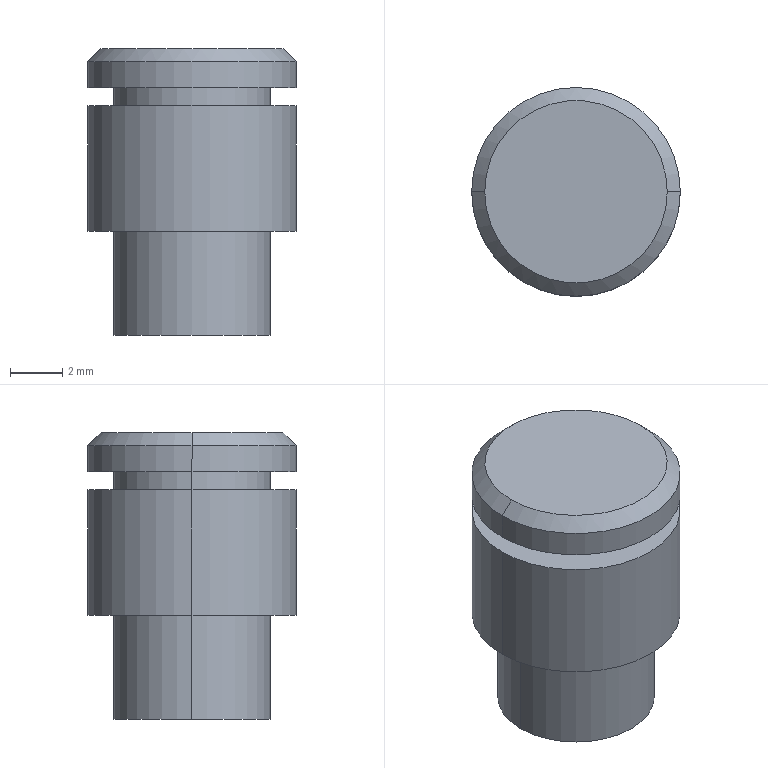Part | STEP file | 8XS200018 | 1 solid | 15 faces | box 8 x 8 x 11 mm | volume 446.551 mm3 | cylinder 8 | plane 5 | cone 2 | commonest cylinder face diameters 6 x4 8 x4
STEP:
#1=CARTESIAN_POINT('',(0.,0.,0.));
#2=DIRECTION('',(0.,0.,1.));
#3=DIRECTION('',(1.,0.,0.));
#4=AXIS2_PLACEMENT_3D('',#1,#2,#3);
#5=CARTESIAN_POINT('',(4.,0.,4.));
#6=VERTEX_POINT('',#5);
#7=CARTESIAN_POINT('',(-4.,0.,4.));
#8=VERTEX_POINT('',#7);
#9=CARTESIAN_POINT('',(0.,0.,4.));
#10=DIRECTION('',(0.,0.,1.));
#11=DIRECTION('',(1.,0.,0.));
#12=AXIS2_PLACEMENT_3D('',#9,#10,#11);
#13=CIRCLE('',#12,4.);
#14=CARTESIAN_POINT('',(0.,0.,0.));
#15=DIRECTION('',(0.,0.,1.));
#16=DIRECTION('',(1.,0.,0.));
#17=AXIS2_PLACEMENT_3D('',#14,#15,#16);
#18=CYLINDRICAL_SURFACE('',#17,4.);
#19=CARTESIAN_POINT('',(0.,4.));
#20=DIRECTION('',(1.,0.));
#21=VECTOR('',#20,1.);
#22=LINE('',#19,#21);
#23=(GEOMETRIC_REPRESENTATION_CONTEXT(2)PARAMETRIC_REPRESENTATION_CONTEXT()REPRESENTATION_CONTEXT('',''));
#24=DEFINITIONAL_REPRESENTATION('',(#22),#23);
#25=PCURVE('',#18,#24);
#26=CARTESIAN_POINT('',(0.,3.5,4.));
#27=DIRECTION('',(0.,0.,1.));
#28=DIRECTION('',(1.,0.,0.));
#29=AXIS2_PLACEMENT_3D('',#26,#27,#28);
#30=PLANE('',#29);
#31=CARTESIAN_POINT('',(0.,-3.5));
#32=DIRECTION('',(1.,0.));
#33=AXIS2_PLACEMENT_2D('',#31,#32);
#34=CIRCLE('',#33,4.);
#35=(GEOMETRIC_REPRESENTATION_CONTEXT(2)PARAMETRIC_REPRESENTATION_CONTEXT()REPRESENTATION_CONTEXT('',''));
#36=DEFINITIONAL_REPRESENTATION('',(#34),#35);
#37=PCURVE('',#30,#36);
#38=SURFACE_CURVE('',#13,(#25,#37),.PCURVE_S1.);
#39=EDGE_CURVE('',#6,#8,#38,.T.);
#40=ORIENTED_EDGE('',*,*,#39,.T.);
#41=CARTESIAN_POINT('',(-4.,0.,8.8));
#42=VERTEX_POINT('',#41);
#43=CARTESIAN_POINT('',(-4.,0.,0.));
#44=DIRECTION('',(0.,0.,1.));
#45=VECTOR('',#44,1.);
#46=LINE('',#43,#45);
#47=CARTESIAN_POINT('',(3.142,0.));
#48=DIRECTION('',(0.,1.));
#49=VECTOR('',#48,1.);
#50=LINE('',#47,#49);
#51=(GEOMETRIC_REPRESENTATION_CONTEXT(2)PARAMETRIC_REPRESENTATION_CONTEXT()REPRESENTATION_CONTEXT('',''));
#52=DEFINITIONAL_REPRESENTATION('',(#50),#51);
#53=PCURVE('',#18,#52);
#54=CARTESIAN_POINT('',(0.,0.,0.));
#55=DIRECTION('',(0.,0.,1.));
#56=DIRECTION('',(1.,0.,0.));
#57=AXIS2_PLACEMENT_3D('',#54,#55,#56);
#58=CYLINDRICAL_SURFACE('',#57,4.);
#59=CARTESIAN_POINT('',(3.142,0.));
#60=DIRECTION('',(0.,1.));
#61=VECTOR('',#60,1.);
#62=LINE('',#59,#61);
#63=(GEOMETRIC_REPRESENTATION_CONTEXT(2)PARAMETRIC_REPRESENTATION_CONTEXT()REPRESENTATION_CONTEXT('',''));
#64=DEFINITIONAL_REPRESENTATION('',(#62),#63);
#65=PCURVE('',#58,#64);
#66=SURFACE_CURVE('',#46,(#53,#65),.PCURVE_S1.);
#67=EDGE_CURVE('',#8,#42,#66,.T.);
#68=ORIENTED_EDGE('',*,*,#67,.T.);
#69=CARTESIAN_POINT('',(4.,0.,8.8));
#70=VERTEX_POINT('',#69);
#71=CARTESIAN_POINT('',(0.,0.,8.8));
#72=DIRECTION('',(0.,0.,-1.));
#73=DIRECTION('',(1.,0.,0.));
#74=AXIS2_PLACEMENT_3D('',#71,#72,#73);
#75=CIRCLE('',#74,4.);
#76=CARTESIAN_POINT('',(6.283,8.8));
#77=DIRECTION('',(-1.,0.));
#78=VECTOR('',#77,1.);
#79=LINE('',#76,#78);
#80=(GEOMETRIC_REPRESENTATION_CONTEXT(2)PARAMETRIC_REPRESENTATION_CONTEXT()REPRESENTATION_CONTEXT('',''));
#81=DEFINITIONAL_REPRESENTATION('',(#79),#80);
#82=PCURVE('',#18,#81);
#83=CARTESIAN_POINT('',(0.,3.5,8.8));
#84=DIRECTION('',(0.,0.,-1.));
#85=DIRECTION('',(-1.,0.,0.));
#86=AXIS2_PLACEMENT_3D('',#83,#84,#85);
#87=PLANE('',#86);
#88=CARTESIAN_POINT('',(0.,-3.5));
#89=DIRECTION('',(-1.,0.));
#90=AXIS2_PLACEMENT_2D('',#88,#89);
#91=CIRCLE('',#90,4.);
#92=(GEOMETRIC_REPRESENTATION_CONTEXT(2)PARAMETRIC_REPRESENTATION_CONTEXT()REPRESENTATION_CONTEXT('',''));
#93=DEFINITIONAL_REPRESENTATION('',(#91),#92);
#94=PCURVE('',#87,#93);
#95=SURFACE_CURVE('',#75,(#82,#94),.PCURVE_S1.);
#96=EDGE_CURVE('',#42,#70,#95,.T.);
#97=ORIENTED_EDGE('',*,*,#96,.T.);
#98=CARTESIAN_POINT('',(4.,0.,0.));
#99=DIRECTION('',(0.,0.,1.));
#100=VECTOR('',#99,1.);
#101=LINE('',#98,#100);
#102=CARTESIAN_POINT('',(0.,0.));
#103=DIRECTION('',(0.,1.));
#104=VECTOR('',#103,1.);
#105=LINE('',#102,#104);
#106=(GEOMETRIC_REPRESENTATION_CONTEXT(2)PARAMETRIC_REPRESENTATION_CONTEXT()REPRESENTATION_CONTEXT('',''));
#107=DEFINITIONAL_REPRESENTATION('',(#105),#106);
#108=PCURVE('',#18,#107);
#109=CARTESIAN_POINT('',(6.283,0.));
#110=DIRECTION('',(0.,1.));
#111=VECTOR('',#110,1.);
#112=LINE('',#109,#111);
#113=(GEOMETRIC_REPRESENTATION_CONTEXT(2)PARAMETRIC_REPRESENTATION_CONTEXT()REPRESENTATION_CONTEXT('',''));
#114=DEFINITIONAL_REPRESENTATION('',(#112),#113);
#115=PCURVE('',#58,#114);
#116=SURFACE_CURVE('',#101,(#108,#115),.PCURVE_S1.);
#117=EDGE_CURVE('',#6,#70,#116,.T.);
#118=ORIENTED_EDGE('',*,*,#117,.F.);
#119=EDGE_LOOP('',(#40,#68,#97,#118));
#120=FACE_BOUND('',#119,.T.);
#121=ADVANCED_FACE('',(#120),#18,.T.);
#122=CARTESIAN_POINT('',(3.,0.,0.));
#123=VERTEX_POINT('',#122);
#124=CARTESIAN_POINT('',(-3.,0.,0.));
#125=VERTEX_POINT('',#124);
#126=CARTESIAN_POINT('',(0.,0.,0.));
#127=DIRECTION('',(0.,0.,1.));
#128=DIRECTION('',(1.,0.,0.));
#129=AXIS2_PLACEMENT_3D('',#126,#127,#128);
#130=CIRCLE('',#129,3.);
#131=CARTESIAN_POINT('',(0.,0.,2.));
#132=DIRECTION('',(0.,0.,1.));
#133=DIRECTION('',(1.,0.,0.));
#134=AXIS2_PLACEMENT_3D('',#131,#132,#133);
#135=CYLINDRICAL_SURFACE('',#134,3.);
#136=CARTESIAN_POINT('',(0.,-2.));
#137=DIRECTION('',(1.,0.));
#138=VECTOR('',#137,1.);
#139=LINE('',#136,#138);
#140=(GEOMETRIC_REPRESENTATION_CONTEXT(2)PARAMETRIC_REPRESENTATION_CONTEXT()REPRESENTATION_CONTEXT('',''));
#141=DEFINITIONAL_REPRESENTATION('',(#139),#140);
#142=PCURVE('',#135,#141);
#143=CARTESIAN_POINT('',(0.,0.,0.));
#144=DIRECTION('',(0.,0.,-1.));
#145=DIRECTION('',(-1.,0.,0.));
#146=AXIS2_PLACEMENT_3D('',#143,#144,#145);
#147=PLANE('',#146);
#148=CARTESIAN_POINT('',(-3.,0.));
#149=CARTESIAN_POINT('',(-3.,5.196));
#150=CARTESIAN_POINT('',(1.5,2.598));
#151=CARTESIAN_POINT('',(6.,0.));
#152=CARTESIAN_POINT('',(1.5,-2.598));
#153=CARTESIAN_POINT('',(-3.,-5.196));
#154=CARTESIAN_POINT('',(-3.,0.));
#155=(BOUNDED_CURVE()B_SPLINE_CURVE(2,(#148,#149,#150,#151,#152,#153,#154),.UNSPECIFIED.,.T.,.F.)B_SPLINE_CURVE_WITH_KNOTS((1,2,2,2,2,1),(-2.094,0.,2.094,4.189,6.283,8.378),.UNSPECIFIED.)CURVE()GEOMETRIC_REPRESENTATION_ITEM()RATIONAL_B_SPLINE_CURVE((1.,0.5,1.,0.5,1.,0.5,1.))REPRESENTATION_ITEM(''));
#156=(GEOMETRIC_REPRESENTATION_CONTEXT(2)PARAMETRIC_REPRESENTATION_CONTEXT()REPRESENTATION_CONTEXT('',''));
#157=DEFINITIONAL_REPRESENTATION('',(#155),#156);
#158=PCURVE('',#147,#157);
#159=SURFACE_CURVE('',#130,(#142,#158),.PCURVE_S1.);
#160=EDGE_CURVE('',#123,#125,#159,.T.);
#161=ORIENTED_EDGE('',*,*,#160,.T.);
#162=CARTESIAN_POINT('',(-3.,0.,4.));
#163=VERTEX_POINT('',#162);
#164=CARTESIAN_POINT('',(-3.,0.,2.));
#165=DIRECTION('',(0.,0.,1.));
#166=VECTOR('',#165,1.);
#167=LINE('',#164,#166);
#168=CARTESIAN_POINT('',(3.142,0.));
#169=DIRECTION('',(0.,1.));
#170=VECTOR('',#169,1.);
#171=LINE('',#168,#170);
#172=(GEOMETRIC_REPRESENTATION_CONTEXT(2)PARAMETRIC_REPRESENTATION_CONTEXT()REPRESENTATION_CONTEXT('',''));
#173=DEFINITIONAL_REPRESENTATION('',(#171),#172);
#174=PCURVE('',#135,#173);
#175=CARTESIAN_POINT('',(0.,0.,2.));
#176=DIRECTION('',(0.,0.,1.));
#177=DIRECTION('',(1.,0.,0.));
#178=AXIS2_PLACEMENT_3D('',#175,#176,#177);
#179=CYLINDRICAL_SURFACE('',#178,3.);
#180=CARTESIAN_POINT('',(3.142,0.));
#181=DIRECTION('',(0.,1.));
#182=VECTOR('',#181,1.);
#183=LINE('',#180,#182);
#184=(GEOMETRIC_REPRESENTATION_CONTEXT(2)PARAMETRIC_REPRESENTATION_CONTEXT()REPRESENTATION_CONTEXT('',''));
#185=DEFINITIONAL_REPRESENTATION('',(#183),#184);
#186=PCURVE('',#179,#185);
#187=SURFACE_CURVE('',#167,(#174,#186),.PCURVE_S1.);
#188=EDGE_CURVE('',#125,#163,#187,.T.);
#189=ORIENTED_EDGE('',*,*,#188,.T.);
#190=CARTESIAN_POINT('',(3.,0.,4.));
#191=VERTEX_POINT('',#190);
#192=CARTESIAN_POINT('',(0.,0.,4.));
#193=DIRECTION('',(0.,0.,-1.));
#194=DIRECTION('',(1.,0.,0.));
#195=AXIS2_PLACEMENT_3D('',#192,#193,#194);
#196=CIRCLE('',#195,3.);
#197=CARTESIAN_POINT('',(6.283,2.));
#198=DIRECTION('',(-1.,0.));
#199=VECTOR('',#198,1.);
#200=LINE('',#197,#199);
#201=(GEOMETRIC_REPRESENTATION_CONTEXT(2)PARAMETRIC_REPRESENTATION_CONTEXT()REPRESENTATION_CONTEXT('',''));
#202=DEFINITIONAL_REPRESENTATION('',(#200),#201);
#203=PCURVE('',#135,#202);
#204=CARTESIAN_POINT('',(3.,-3.5));
#205=CARTESIAN_POINT('',(3.,-8.696));
#206=CARTESIAN_POINT('',(-1.5,-6.098));
#207=CARTESIAN_POINT('',(-6.,-3.5));
#208=CARTESIAN_POINT('',(-1.5,-0.9019));
#209=CARTESIAN_POINT('',(3.,1.696));
#210=CARTESIAN_POINT('',(3.,-3.5));
#211=(BOUNDED_CURVE()B_SPLINE_CURVE(2,(#204,#205,#206,#207,#208,#209,#210),.UNSPECIFIED.,.T.,.F.)B_SPLINE_CURVE_WITH_KNOTS((1,2,2,2,2,1),(-2.094,0.,2.094,4.189,6.283,8.378),.UNSPECIFIED.)CURVE()GEOMETRIC_REPRESENTATION_ITEM()RATIONAL_B_SPLINE_CURVE((1.,0.5,1.,0.5,1.,0.5,1.))REPRESENTATION_ITEM(''));
#212=(GEOMETRIC_REPRESENTATION_CONTEXT(2)PARAMETRIC_REPRESENTATION_CONTEXT()REPRESENTATION_CONTEXT('',''));
#213=DEFINITIONAL_REPRESENTATION('',(#211),#212);
#214=PCURVE('',#30,#213);
#215=SURFACE_CURVE('',#196,(#203,#214),.PCURVE_S1.);
#216=EDGE_CURVE('',#163,#191,#215,.T.);
#217=ORIENTED_EDGE('',*,*,#216,.T.);
#218=CARTESIAN_POINT('',(3.,0.,2.));
#219=DIRECTION('',(0.,0.,1.));
#220=VECTOR('',#219,1.);
#221=LINE('',#218,#220);
#222=CARTESIAN_POINT('',(0.,0.));
#223=DIRECTION('',(0.,1.));
#224=VECTOR('',#223,1.);
#225=LINE('',#222,#224);
#226=(GEOMETRIC_REPRESENTATION_CONTEXT(2)PARAMETRIC_REPRESENTATION_CONTEXT()REPRESENTATION_CONTEXT('',''));
#227=DEFINITIONAL_REPRESENTATION('',(#225),#226);
#228=PCURVE('',#135,#227);
#229=CARTESIAN_POINT('',(6.283,0.));
#230=DIRECTION('',(0.,1.));
#231=VECTOR('',#230,1.);
#232=LINE('',#229,#231);
#233=(GEOMETRIC_REPRESENTATION_CONTEXT(2)PARAMETRIC_REPRESENTATION_CONTEXT()REPRESENTATION_CONTEXT('',''));
#234=DEFINITIONAL_REPRESENTATION('',(#232),#233);
#235=PCURVE('',#179,#234);
#236=SURFACE_CURVE('',#221,(#228,#235),.PCURVE_S1.);
#237=EDGE_CURVE('',#123,#191,#236,.T.);
#238=ORIENTED_EDGE('',*,*,#237,.F.);
#239=EDGE_LOOP('',(#161,#189,#217,#238));
#240=FACE_BOUND('',#239,.T.);
#241=ADVANCED_FACE('',(#240),#135,.T.);
#242=CARTESIAN_POINT('',(3.,0.,8.8));
#243=VERTEX_POINT('',#242);
#244=CARTESIAN_POINT('',(-3.,0.,8.8));
#245=VERTEX_POINT('',#244);
#246=CARTESIAN_POINT('',(0.,0.,8.8));
#247=DIRECTION('',(0.,0.,1.));
#248=DIRECTION('',(1.,0.,0.));
#249=AXIS2_PLACEMENT_3D('',#246,#247,#248);
#250=CIRCLE('',#249,3.);
#251=CARTESIAN_POINT('',(0.,0.,9.15));
#252=DIRECTION('',(0.,0.,1.));
#253=DIRECTION('',(1.,0.,0.));
#254=AXIS2_PLACEMENT_3D('',#251,#252,#253);
#255=CYLINDRICAL_SURFACE('',#254,3.);
#256=CARTESIAN_POINT('',(0.,-0.35));
#257=DIRECTION('',(1.,0.));
#258=VECTOR('',#257,1.);
#259=LINE('',#256,#258);
#260=(GEOMETRIC_REPRESENTATION_CONTEXT(2)PARAMETRIC_REPRESENTATION_CONTEXT()REPRESENTATION_CONTEXT('',''));
#261=DEFINITIONAL_REPRESENTATION('',(#259),#260);
#262=PCURVE('',#255,#261);
#263=CARTESIAN_POINT('',(-3.,-3.5));
#264=CARTESIAN_POINT('',(-3.,1.696));
#265=CARTESIAN_POINT('',(1.5,-0.9019));
#266=CARTESIAN_POINT('',(6.,-3.5));
#267=CARTESIAN_POINT('',(1.5,-6.098));
#268=CARTESIAN_POINT('',(-3.,-8.696));
#269=CARTESIAN_POINT('',(-3.,-3.5));
#270=(BOUNDED_CURVE()B_SPLINE_CURVE(2,(#263,#264,#265,#266,#267,#268,#269),.UNSPECIFIED.,.T.,.F.)B_SPLINE_CURVE_WITH_KNOTS((1,2,2,2,2,1),(-2.094,0.,2.094,4.189,6.283,8.378),.UNSPECIFIED.)CURVE()GEOMETRIC_REPRESENTATION_ITEM()RATIONAL_B_SPLINE_CURVE((1.,0.5,1.,0.5,1.,0.5,1.))REPRESENTATION_ITEM(''));
#271=(GEOMETRIC_REPRESENTATION_CONTEXT(2)PARAMETRIC_REPRESENTATION_CONTEXT()REPRESENTATION_CONTEXT('',''));
#272=DEFINITIONAL_REPRESENTATION('',(#270),#271);
#273=PCURVE('',#87,#272);
#274=SURFACE_CURVE('',#250,(#262,#273),.PCURVE_S1.);
#275=EDGE_CURVE('',#243,#245,#274,.T.);
#276=ORIENTED_EDGE('',*,*,#275,.T.);
#277=CARTESIAN_POINT('',(-3.,0.,9.5));
#278=VERTEX_POINT('',#277);
#279=CARTESIAN_POINT('',(-3.,0.,9.15));
#280=DIRECTION('',(0.,0.,1.));
#281=VECTOR('',#280,1.);
#282=LINE('',#279,#281);
#283=CARTESIAN_POINT('',(3.142,0.));
#284=DIRECTION('',(0.,1.));
#285=VECTOR('',#284,1.);
#286=LINE('',#283,#285);
#287=(GEOMETRIC_REPRESENTATION_CONTEXT(2)PARAMETRIC_REPRESENTATION_CONTEXT()REPRESENTATION_CONTEXT('',''));
#288=DEFINITIONAL_REPRESENTATION('',(#286),#287);
#289=PCURVE('',#255,#288);
#290=CARTESIAN_POINT('',(0.,0.,9.15));
#291=DIRECTION('',(0.,0.,1.));
#292=DIRECTION('',(1.,0.,0.));
#293=AXIS2_PLACEMENT_3D('',#290,#291,#292);
#294=CYLINDRICAL_SURFACE('',#293,3.);
#295=CARTESIAN_POINT('',(3.142,0.));
#296=DIRECTION('',(0.,1.));
#297=VECTOR('',#296,1.);
#298=LINE('',#295,#297);
#299=(GEOMETRIC_REPRESENTATION_CONTEXT(2)PARAMETRIC_REPRESENTATION_CONTEXT()REPRESENTATION_CONTEXT('',''));
#300=DEFINITIONAL_REPRESENTATION('',(#298),#299);
#301=PCURVE('',#294,#300);
#302=SURFACE_CURVE('',#282,(#289,#301),.PCURVE_S1.);
#303=EDGE_CURVE('',#245,#278,#302,.T.);
#304=ORIENTED_EDGE('',*,*,#303,.T.);
#305=CARTESIAN_POINT('',(3.,0.,9.5));
#306=VERTEX_POINT('',#305);
#307=CARTESIAN_POINT('',(0.,0.,9.5));
#308=DIRECTION('',(0.,0.,-1.));
#309=DIRECTION('',(1.,0.,0.));
#310=AXIS2_PLACEMENT_3D('',#307,#308,#309);
#311=CIRCLE('',#310,3.);
#312=CARTESIAN_POINT('',(6.283,0.35));
#313=DIRECTION('',(-1.,0.));
#314=VECTOR('',#313,1.);
#315=LINE('',#312,#314);
#316=(GEOMETRIC_REPRESENTATION_CONTEXT(2)PARAMETRIC_REPRESENTATION_CONTEXT()REPRESENTATION_CONTEXT('',''));
#317=DEFINITIONAL_REPRESENTATION('',(#315),#316);
#318=PCURVE('',#255,#317);
#319=CARTESIAN_POINT('',(0.,3.5,9.5));
#320=DIRECTION('',(0.,0.,1.));
#321=DIRECTION('',(1.,0.,0.));
#322=AXIS2_PLACEMENT_3D('',#319,#320,#321);
#323=PLANE('',#322);
#324=CARTESIAN_POINT('',(3.,-3.5));
#325=CARTESIAN_POINT('',(3.,-8.696));
#326=CARTESIAN_POINT('',(-1.5,-6.098));
#327=CARTESIAN_POINT('',(-6.,-3.5));
#328=CARTESIAN_POINT('',(-1.5,-0.9019));
#329=CARTESIAN_POINT('',(3.,1.696));
#330=CARTESIAN_POINT('',(3.,-3.5));
#331=(BOUNDED_CURVE()B_SPLINE_CURVE(2,(#324,#325,#326,#327,#328,#329,#330),.UNSPECIFIED.,.T.,.F.)B_SPLINE_CURVE_WITH_KNOTS((1,2,2,2,2,1),(-2.094,0.,2.094,4.189,6.283,8.378),.UNSPECIFIED.)CURVE()GEOMETRIC_REPRESENTATION_ITEM()RATIONAL_B_SPLINE_CURVE((1.,0.5,1.,0.5,1.,0.5,1.))REPRESENTATION_ITEM(''));
#332=(GEOMETRIC_REPRESENTATION_CONTEXT(2)PARAMETRIC_REPRESENTATION_CONTEXT()REPRESENTATION_CONTEXT('',''));
#333=DEFINITIONAL_REPRESENTATION('',(#331),#332);
#334=PCURVE('',#323,#333);
#335=SURFACE_CURVE('',#311,(#318,#334),.PCURVE_S1.);
#336=EDGE_CURVE('',#278,#306,#335,.T.);
#337=ORIENTED_EDGE('',*,*,#336,.T.);
#338=CARTESIAN_POINT('',(3.,0.,9.15));
#339=DIRECTION('',(0.,0.,1.));
#340=VECTOR('',#339,1.);
#341=LINE('',#338,#340);
#342=CARTESIAN_POINT('',(0.,0.));
#343=DIRECTION('',(0.,1.));
#344=VECTOR('',#343,1.);
#345=LINE('',#342,#344);
#346=(GEOMETRIC_REPRESENTATION_CONTEXT(2)PARAMETRIC_REPRESENTATION_CONTEXT()REPRESENTATION_CONTEXT('',''));
#347=DEFINITIONAL_REPRESENTATION('',(#345),#346);
#348=PCURVE('',#255,#347);
#349=CARTESIAN_POINT('',(6.283,0.));
#350=DIRECTION('',(0.,1.));
#351=VECTOR('',#350,1.);
#352=LINE('',#349,#351);
#353=(GEOMETRIC_REPRESENTATION_CONTEXT(2)PARAMETRIC_REPRESENTATION_CONTEXT()REPRESENTATION_CONTEXT('',''));
#354=DEFINITIONAL_REPRESENTATION('',(#352),#353);
#355=PCURVE('',#294,#354);
#356=SURFACE_CURVE('',#341,(#348,#355),.PCURVE_S1.);
#357=EDGE_CURVE('',#243,#306,#356,.T.);
#358=ORIENTED_EDGE('',*,*,#357,.F.);
#359=EDGE_LOOP('',(#276,#304,#337,#358));
#360=FACE_BOUND('',#359,.T.);
#361=ADVANCED_FACE('',(#360),#255,.T.);
#362=CARTESIAN_POINT('',(4.,0.,9.5));
#363=VERTEX_POINT('',#362);
#364=CARTESIAN_POINT('',(-4.,0.,9.5));
#365=VERTEX_POINT('',#364);
#366=CARTESIAN_POINT('',(0.,0.,9.5));
#367=DIRECTION('',(0.,0.,1.));
#368=DIRECTION('',(1.,0.,0.));
#369=AXIS2_PLACEMENT_3D('',#366,#367,#368);
#370=CIRCLE('',#369,4.);
#371=CARTESIAN_POINT('',(0.,0.,0.));
#372=DIRECTION('',(0.,0.,1.));
#373=DIRECTION('',(1.,0.,0.));
#374=AXIS2_PLACEMENT_3D('',#371,#372,#373);
#375=CYLINDRICAL_SURFACE('',#374,4.);
#376=CARTESIAN_POINT('',(0.,9.5));
#377=DIRECTION('',(1.,0.));
#378=VECTOR('',#377,1.);
#379=LINE('',#376,#378);
#380=(GEOMETRIC_REPRESENTATION_CONTEXT(2)PARAMETRIC_REPRESENTATION_CONTEXT()REPRESENTATION_CONTEXT('',''));
#381=DEFINITIONAL_REPRESENTATION('',(#379),#380);
#382=PCURVE('',#375,#381);
#383=CARTESIAN_POINT('',(0.,-3.5));
#384=DIRECTION('',(1.,0.));
#385=AXIS2_PLACEMENT_2D('',#383,#384);
#386=CIRCLE('',#385,4.);
#387=(GEOMETRIC_REPRESENTATION_CONTEXT(2)PARAMETRIC_REPRESENTATION_CONTEXT()REPRESENTATION_CONTEXT('',''));
#388=DEFINITIONAL_REPRESENTATION('',(#386),#387);
#389=PCURVE('',#323,#388);
#390=SURFACE_CURVE('',#370,(#382,#389),.PCURVE_S1.);
#391=EDGE_CURVE('',#363,#365,#390,.T.);
#392=ORIENTED_EDGE('',*,*,#391,.T.);
#393=CARTESIAN_POINT('',(-4.,0.,10.5));
#394=VERTEX_POINT('',#393);
#395=CARTESIAN_POINT('',(-4.,0.,0.));
#396=DIRECTION('',(0.,0.,1.));
#397=VECTOR('',#396,1.);
#398=LINE('',#395,#397);
#399=CARTESIAN_POINT('',(3.142,0.));
#400=DIRECTION('',(0.,1.));
#401=VECTOR('',#400,1.);
#402=LINE('',#399,#401);
#403=(GEOMETRIC_REPRESENTATION_CONTEXT(2)PARAMETRIC_REPRESENTATION_CONTEXT()REPRESENTATION_CONTEXT('',''));
#404=DEFINITIONAL_REPRESENTATION('',(#402),#403);
#405=PCURVE('',#375,#404);
#406=CARTESIAN_POINT('',(0.,0.,0.));
#407=DIRECTION('',(0.,0.,1.));
#408=DIRECTION('',(1.,0.,0.));
#409=AXIS2_PLACEMENT_3D('',#406,#407,#408);
#410=CYLINDRICAL_SURFACE('',#409,4.);
#411=CARTESIAN_POINT('',(3.142,0.));
#412=DIRECTION('',(0.,1.));
#413=VECTOR('',#412,1.);
#414=LINE('',#411,#413);
#415=(GEOMETRIC_REPRESENTATION_CONTEXT(2)PARAMETRIC_REPRESENTATION_CONTEXT()REPRESENTATION_CONTEXT('',''));
#416=DEFINITIONAL_REPRESENTATION('',(#414),#415);
#417=PCURVE('',#410,#416);
#418=SURFACE_CURVE('',#398,(#405,#417),.PCURVE_S1.);
#419=EDGE_CURVE('',#365,#394,#418,.T.);
#420=ORIENTED_EDGE('',*,*,#419,.T.);
#421=CARTESIAN_POINT('',(4.,0.,10.5));
#422=VERTEX_POINT('',#421);
#423=CARTESIAN_POINT('',(0.,0.,10.5));
#424=DIRECTION('',(0.,0.,-1.));
#425=DIRECTION('',(1.,0.,0.));
#426=AXIS2_PLACEMENT_3D('',#423,#424,#425);
#427=CIRCLE('',#426,4.);
#428=CARTESIAN_POINT('',(6.283,10.5));
#429=DIRECTION('',(-1.,0.));
#430=VECTOR('',#429,1.);
#431=LINE('',#428,#430);
#432=(GEOMETRIC_REPRESENTATION_CONTEXT(2)PARAMETRIC_REPRESENTATION_CONTEXT()REPRESENTATION_CONTEXT('',''));
#433=DEFINITIONAL_REPRESENTATION('',(#431),#432);
#434=PCURVE('',#375,#433);
#435=CARTESIAN_POINT('',(0.,0.,10.5));
#436=DIRECTION('',(0.,0.,-1.));
#437=DIRECTION('',(-1.,0.,0.));
#438=AXIS2_PLACEMENT_3D('',#435,#436,#437);
#439=CONICAL_SURFACE('',#438,4.,0.7854);
#440=CARTESIAN_POINT('',(-3.142,0.));
#441=DIRECTION('',(1.,0.));
#442=VECTOR('',#441,1.);
#443=LINE('',#440,#442);
#444=(GEOMETRIC_REPRESENTATION_CONTEXT(2)PARAMETRIC_REPRESENTATION_CONTEXT()REPRESENTATION_CONTEXT('',''));
#445=DEFINITIONAL_REPRESENTATION('',(#443),#444);
#446=PCURVE('',#439,#445);
#447=SURFACE_CURVE('',#427,(#434,#446),.PCURVE_S1.);
#448=EDGE_CURVE('',#394,#422,#447,.T.);
#449=ORIENTED_EDGE('',*,*,#448,.T.);
#450=CARTESIAN_POINT('',(4.,0.,0.));
#451=DIRECTION('',(0.,0.,1.));
#452=VECTOR('',#451,1.);
#453=LINE('',#450,#452);
#454=CARTESIAN_POINT('',(0.,0.));
#455=DIRECTION('',(0.,1.));
#456=VECTOR('',#455,1.);
#457=LINE('',#454,#456);
#458=(GEOMETRIC_REPRESENTATION_CONTEXT(2)PARAMETRIC_REPRESENTATION_CONTEXT()REPRESENTATION_CONTEXT('',''));
#459=DEFINITIONAL_REPRESENTATION('',(#457),#458);
#460=PCURVE('',#375,#459);
#461=CARTESIAN_POINT('',(6.283,0.));
#462=DIRECTION('',(0.,1.));
#463=VECTOR('',#462,1.);
#464=LINE('',#461,#463);
#465=(GEOMETRIC_REPRESENTATION_CONTEXT(2)PARAMETRIC_REPRESENTATION_CONTEXT()REPRESENTATION_CONTEXT('',''));
#466=DEFINITIONAL_REPRESENTATION('',(#464),#465);
#467=PCURVE('',#410,#466);
#468=SURFACE_CURVE('',#453,(#460,#467),.PCURVE_S1.);
#469=EDGE_CURVE('',#363,#422,#468,.T.);
#470=ORIENTED_EDGE('',*,*,#469,.F.);
#471=EDGE_LOOP('',(#392,#420,#449,#470));
#472=FACE_BOUND('',#471,.T.);
#473=ADVANCED_FACE('',(#472),#375,.T.);
#474=CARTESIAN_POINT('',(-3.5,0.,11.));
#475=VERTEX_POINT('',#474);
#476=CARTESIAN_POINT('',(3.5,0.,11.));
#477=VERTEX_POINT('',#476);
#478=CARTESIAN_POINT('',(0.,0.,11.));
#479=DIRECTION('',(0.,0.,-1.));
#480=DIRECTION('',(-1.,0.,0.));
#481=AXIS2_PLACEMENT_3D('',#478,#479,#480);
#482=CIRCLE('',#481,3.5);
#483=CARTESIAN_POINT('',(0.,-0.5));
#484=DIRECTION('',(1.,0.));
#485=VECTOR('',#484,1.);
#486=LINE('',#483,#485);
#487=(GEOMETRIC_REPRESENTATION_CONTEXT(2)PARAMETRIC_REPRESENTATION_CONTEXT()REPRESENTATION_CONTEXT('',''));
#488=DEFINITIONAL_REPRESENTATION('',(#486),#487);
#489=PCURVE('',#439,#488);
#490=CARTESIAN_POINT('',(0.,0.,11.));
#491=DIRECTION('',(0.,0.,-1.));
#492=DIRECTION('',(-1.,0.,0.));
#493=AXIS2_PLACEMENT_3D('',#490,#491,#492);
#494=PLANE('',#493);
#495=CARTESIAN_POINT('',(0.,0.));
#496=DIRECTION('',(1.,0.));
#497=AXIS2_PLACEMENT_2D('',#495,#496);
#498=CIRCLE('',#497,3.5);
#499=(GEOMETRIC_REPRESENTATION_CONTEXT(2)PARAMETRIC_REPRESENTATION_CONTEXT()REPRESENTATION_CONTEXT('',''));
#500=DEFINITIONAL_REPRESENTATION('',(#498),#499);
#501=PCURVE('',#494,#500);
#502=SURFACE_CURVE('',#482,(#489,#501),.PCURVE_S1.);
#503=EDGE_CURVE('',#475,#477,#502,.T.);
#504=ORIENTED_EDGE('',*,*,#503,.T.);
#505=CARTESIAN_POINT('',(4.,0.,10.5));
#506=DIRECTION('',(0.7071,0.,-0.7071));
#507=VECTOR('',#506,1.);
#508=LINE('',#505,#507);
#509=CARTESIAN_POINT('',(3.142,0.));
#510=DIRECTION('',(0.,1.));
#511=VECTOR('',#510,1.);
#512=LINE('',#509,#511);
#513=(GEOMETRIC_REPRESENTATION_CONTEXT(2)PARAMETRIC_REPRESENTATION_CONTEXT()REPRESENTATION_CONTEXT('',''));
#514=DEFINITIONAL_REPRESENTATION('',(#512),#513);
#515=PCURVE('',#439,#514);
#516=CARTESIAN_POINT('',(0.,0.,10.5));
#517=DIRECTION('',(0.,0.,-1.));
#518=DIRECTION('',(-1.,0.,0.));
#519=AXIS2_PLACEMENT_3D('',#516,#517,#518);
#520=CONICAL_SURFACE('',#519,4.,0.7854);
#521=CARTESIAN_POINT('',(3.142,0.));
#522=DIRECTION('',(0.,1.));
#523=VECTOR('',#522,1.);
#524=LINE('',#521,#523);
#525=(GEOMETRIC_REPRESENTATION_CONTEXT(2)PARAMETRIC_REPRESENTATION_CONTEXT()REPRESENTATION_CONTEXT('',''));
#526=DEFINITIONAL_REPRESENTATION('',(#524),#525);
#527=PCURVE('',#520,#526);
#528=SURFACE_CURVE('',#508,(#515,#527),.PCURVE_S1.);
#529=EDGE_CURVE('',#477,#422,#528,.T.);
#530=ORIENTED_EDGE('',*,*,#529,.T.);
#531=ORIENTED_EDGE('',*,*,#448,.F.);
#532=CARTESIAN_POINT('',(-4.,0.,10.5));
#533=DIRECTION('',(-0.7071,0.,-0.7071));
#534=VECTOR('',#533,1.);
#535=LINE('',#532,#534);
#536=CARTESIAN_POINT('',(0.,0.));
#537=DIRECTION('',(0.,1.));
#538=VECTOR('',#537,1.);
#539=LINE('',#536,#538);
#540=(GEOMETRIC_REPRESENTATION_CONTEXT(2)PARAMETRIC_REPRESENTATION_CONTEXT()REPRESENTATION_CONTEXT('',''));
#541=DEFINITIONAL_REPRESENTATION('',(#539),#540);
#542=PCURVE('',#439,#541);
#543=CARTESIAN_POINT('',(6.283,0.));
#544=DIRECTION('',(0.,1.));
#545=VECTOR('',#544,1.);
#546=LINE('',#543,#545);
#547=(GEOMETRIC_REPRESENTATION_CONTEXT(2)PARAMETRIC_REPRESENTATION_CONTEXT()REPRESENTATION_CONTEXT('',''));
#548=DEFINITIONAL_REPRESENTATION('',(#546),#547);
#549=PCURVE('',#520,#548);
#550=SURFACE_CURVE('',#535,(#542,#549),.PCURVE_S1.);
#551=EDGE_CURVE('',#475,#394,#550,.T.);
#552=ORIENTED_EDGE('',*,*,#551,.F.);
#553=EDGE_LOOP('',(#504,#530,#531,#552));
#554=FACE_BOUND('',#553,.T.);
#555=ADVANCED_FACE('',(#554),#439,.T.);
#556=ORIENTED_EDGE('',*,*,#67,.F.);
#557=CARTESIAN_POINT('',(0.,0.,4.));
#558=DIRECTION('',(0.,0.,1.));
#559=DIRECTION('',(1.,0.,0.));
#560=AXIS2_PLACEMENT_3D('',#557,#558,#559);
#561=CIRCLE('',#560,4.);
#562=CARTESIAN_POINT('',(0.,4.));
#563=DIRECTION('',(1.,0.));
#564=VECTOR('',#563,1.);
#565=LINE('',#562,#564);
#566=(GEOMETRIC_REPRESENTATION_CONTEXT(2)PARAMETRIC_REPRESENTATION_CONTEXT()REPRESENTATION_CONTEXT('',''));
#567=DEFINITIONAL_REPRESENTATION('',(#565),#566);
#568=PCURVE('',#58,#567);
#569=CARTESIAN_POINT('',(0.,-3.5));
#570=DIRECTION('',(1.,0.));
#571=AXIS2_PLACEMENT_2D('',#569,#570);
#572=CIRCLE('',#571,4.);
#573=(GEOMETRIC_REPRESENTATION_CONTEXT(2)PARAMETRIC_REPRESENTATION_CONTEXT()REPRESENTATION_CONTEXT('',''));
#574=DEFINITIONAL_REPRESENTATION('',(#572),#573);
#575=PCURVE('',#30,#574);
#576=SURFACE_CURVE('',#561,(#568,#575),.PCURVE_S1.);
#577=EDGE_CURVE('',#8,#6,#576,.T.);
#578=ORIENTED_EDGE('',*,*,#577,.T.);
#579=ORIENTED_EDGE('',*,*,#117,.T.);
#580=CARTESIAN_POINT('',(0.,0.,8.8));
#581=DIRECTION('',(0.,0.,-1.));
#582=DIRECTION('',(1.,0.,0.));
#583=AXIS2_PLACEMENT_3D('',#580,#581,#582);
#584=CIRCLE('',#583,4.);
#585=CARTESIAN_POINT('',(6.283,8.8));
#586=DIRECTION('',(-1.,0.));
#587=VECTOR('',#586,1.);
#588=LINE('',#585,#587);
#589=(GEOMETRIC_REPRESENTATION_CONTEXT(2)PARAMETRIC_REPRESENTATION_CONTEXT()REPRESENTATION_CONTEXT('',''));
#590=DEFINITIONAL_REPRESENTATION('',(#588),#589);
#591=PCURVE('',#58,#590);
#592=CARTESIAN_POINT('',(0.,-3.5));
#593=DIRECTION('',(-1.,0.));
#594=AXIS2_PLACEMENT_2D('',#592,#593);
#595=CIRCLE('',#594,4.);
#596=(GEOMETRIC_REPRESENTATION_CONTEXT(2)PARAMETRIC_REPRESENTATION_CONTEXT()REPRESENTATION_CONTEXT('',''));
#597=DEFINITIONAL_REPRESENTATION('',(#595),#596);
#598=PCURVE('',#87,#597);
#599=SURFACE_CURVE('',#584,(#591,#598),.PCURVE_S1.);
#600=EDGE_CURVE('',#70,#42,#599,.T.);
#601=ORIENTED_EDGE('',*,*,#600,.T.);
#602=EDGE_LOOP('',(#556,#578,#579,#601));
#603=FACE_BOUND('',#602,.T.);
#604=ADVANCED_FACE('',(#603),#58,.T.);
#605=CARTESIAN_POINT('',(0.,0.,4.));
#606=DIRECTION('',(0.,0.,-1.));
#607=DIRECTION('',(1.,0.,0.));
#608=AXIS2_PLACEMENT_3D('',#605,#606,#607);
#609=CIRCLE('',#608,3.);
#610=CARTESIAN_POINT('',(3.,-3.5));
#611=CARTESIAN_POINT('',(3.,-8.696));
#612=CARTESIAN_POINT('',(-1.5,-6.098));
#613=CARTESIAN_POINT('',(-6.,-3.5));
#614=CARTESIAN_POINT('',(-1.5,-0.9019));
#615=CARTESIAN_POINT('',(3.,1.696));
#616=CARTESIAN_POINT('',(3.,-3.5));
#617=(BOUNDED_CURVE()B_SPLINE_CURVE(2,(#610,#611,#612,#613,#614,#615,#616),.UNSPECIFIED.,.T.,.F.)B_SPLINE_CURVE_WITH_KNOTS((1,2,2,2,2,1),(-2.094,0.,2.094,4.189,6.283,8.378),.UNSPECIFIED.)CURVE()GEOMETRIC_REPRESENTATION_ITEM()RATIONAL_B_SPLINE_CURVE((1.,0.5,1.,0.5,1.,0.5,1.))REPRESENTATION_ITEM(''));
#618=(GEOMETRIC_REPRESENTATION_CONTEXT(2)PARAMETRIC_REPRESENTATION_CONTEXT()REPRESENTATION_CONTEXT('',''));
#619=DEFINITIONAL_REPRESENTATION('',(#617),#618);
#620=PCURVE('',#30,#619);
#621=CARTESIAN_POINT('',(6.283,2.));
#622=DIRECTION('',(-1.,0.));
#623=VECTOR('',#622,1.);
#624=LINE('',#621,#623);
#625=(GEOMETRIC_REPRESENTATION_CONTEXT(2)PARAMETRIC_REPRESENTATION_CONTEXT()REPRESENTATION_CONTEXT('',''));
#626=DEFINITIONAL_REPRESENTATION('',(#624),#625);
#627=PCURVE('',#179,#626);
#628=SURFACE_CURVE('',#609,(#620,#627),.PCURVE_S1.);
#629=EDGE_CURVE('',#191,#163,#628,.T.);
#630=ORIENTED_EDGE('',*,*,#629,.F.);
#631=ORIENTED_EDGE('',*,*,#216,.F.);
#632=EDGE_LOOP('',(#630,#631));
#633=FACE_BOUND('',#632,.T.);
#634=ORIENTED_EDGE('',*,*,#39,.F.);
#635=ORIENTED_EDGE('',*,*,#577,.F.);
#636=EDGE_LOOP('',(#634,#635));
#637=FACE_BOUND('',#636,.T.);
#638=ADVANCED_FACE('',(#633,#637),#30,.F.);
#639=ORIENTED_EDGE('',*,*,#275,.F.);
#640=CARTESIAN_POINT('',(0.,0.,8.8));
#641=DIRECTION('',(0.,0.,1.));
#642=DIRECTION('',(1.,0.,0.));
#643=AXIS2_PLACEMENT_3D('',#640,#641,#642);
#644=CIRCLE('',#643,3.);
#645=CARTESIAN_POINT('',(-3.,-3.5));
#646=CARTESIAN_POINT('',(-3.,1.696));
#647=CARTESIAN_POINT('',(1.5,-0.9019));
#648=CARTESIAN_POINT('',(6.,-3.5));
#649=CARTESIAN_POINT('',(1.5,-6.098));
#650=CARTESIAN_POINT('',(-3.,-8.696));
#651=CARTESIAN_POINT('',(-3.,-3.5));
#652=(BOUNDED_CURVE()B_SPLINE_CURVE(2,(#645,#646,#647,#648,#649,#650,#651),.UNSPECIFIED.,.T.,.F.)B_SPLINE_CURVE_WITH_KNOTS((1,2,2,2,2,1),(-2.094,0.,2.094,4.189,6.283,8.378),.UNSPECIFIED.)CURVE()GEOMETRIC_REPRESENTATION_ITEM()RATIONAL_B_SPLINE_CURVE((1.,0.5,1.,0.5,1.,0.5,1.))REPRESENTATION_ITEM(''));
#653=(GEOMETRIC_REPRESENTATION_CONTEXT(2)PARAMETRIC_REPRESENTATION_CONTEXT()REPRESENTATION_CONTEXT('',''));
#654=DEFINITIONAL_REPRESENTATION('',(#652),#653);
#655=PCURVE('',#87,#654);
#656=CARTESIAN_POINT('',(0.,-0.35));
#657=DIRECTION('',(1.,0.));
#658=VECTOR('',#657,1.);
#659=LINE('',#656,#658);
#660=(GEOMETRIC_REPRESENTATION_CONTEXT(2)PARAMETRIC_REPRESENTATION_CONTEXT()REPRESENTATION_CONTEXT('',''));
#661=DEFINITIONAL_REPRESENTATION('',(#659),#660);
#662=PCURVE('',#294,#661);
#663=SURFACE_CURVE('',#644,(#655,#662),.PCURVE_S1.);
#664=EDGE_CURVE('',#245,#243,#663,.T.);
#665=ORIENTED_EDGE('',*,*,#664,.F.);
#666=EDGE_LOOP('',(#639,#665));
#667=FACE_BOUND('',#666,.T.);
#668=ORIENTED_EDGE('',*,*,#600,.F.);
#669=ORIENTED_EDGE('',*,*,#96,.F.);
#670=EDGE_LOOP('',(#668,#669));
#671=FACE_BOUND('',#670,.T.);
#672=ADVANCED_FACE('',(#667,#671),#87,.F.);
#673=ORIENTED_EDGE('',*,*,#188,.F.);
#674=CARTESIAN_POINT('',(0.,0.,0.));
#675=DIRECTION('',(0.,0.,1.));
#676=DIRECTION('',(1.,0.,0.));
#677=AXIS2_PLACEMENT_3D('',#674,#675,#676);
#678=CIRCLE('',#677,3.);
#679=CARTESIAN_POINT('',(0.,-2.));
#680=DIRECTION('',(1.,0.));
#681=VECTOR('',#680,1.);
#682=LINE('',#679,#681);
#683=(GEOMETRIC_REPRESENTATION_CONTEXT(2)PARAMETRIC_REPRESENTATION_CONTEXT()REPRESENTATION_CONTEXT('',''));
#684=DEFINITIONAL_REPRESENTATION('',(#682),#683);
#685=PCURVE('',#179,#684);
#686=CARTESIAN_POINT('',(-3.,0.));
#687=CARTESIAN_POINT('',(-3.,5.196));
#688=CARTESIAN_POINT('',(1.5,2.598));
#689=CARTESIAN_POINT('',(6.,0.));
#690=CARTESIAN_POINT('',(1.5,-2.598));
#691=CARTESIAN_POINT('',(-3.,-5.196));
#692=CARTESIAN_POINT('',(-3.,0.));
#693=(BOUNDED_CURVE()B_SPLINE_CURVE(2,(#686,#687,#688,#689,#690,#691,#692),.UNSPECIFIED.,.T.,.F.)B_SPLINE_CURVE_WITH_KNOTS((1,2,2,2,2,1),(-2.094,0.,2.094,4.189,6.283,8.378),.UNSPECIFIED.)CURVE()GEOMETRIC_REPRESENTATION_ITEM()RATIONAL_B_SPLINE_CURVE((1.,0.5,1.,0.5,1.,0.5,1.))REPRESENTATION_ITEM(''));
#694=(GEOMETRIC_REPRESENTATION_CONTEXT(2)PARAMETRIC_REPRESENTATION_CONTEXT()REPRESENTATION_CONTEXT('',''));
#695=DEFINITIONAL_REPRESENTATION('',(#693),#694);
#696=PCURVE('',#147,#695);
#697=SURFACE_CURVE('',#678,(#685,#696),.PCURVE_S1.);
#698=EDGE_CURVE('',#125,#123,#697,.T.);
#699=ORIENTED_EDGE('',*,*,#698,.T.);
#700=ORIENTED_EDGE('',*,*,#237,.T.);
#701=ORIENTED_EDGE('',*,*,#629,.T.);
#702=EDGE_LOOP('',(#673,#699,#700,#701));
#703=FACE_BOUND('',#702,.T.);
#704=ADVANCED_FACE('',(#703),#179,.T.);
#705=ORIENTED_EDGE('',*,*,#303,.F.);
#706=ORIENTED_EDGE('',*,*,#664,.T.);
#707=ORIENTED_EDGE('',*,*,#357,.T.);
#708=CARTESIAN_POINT('',(0.,0.,9.5));
#709=DIRECTION('',(0.,0.,-1.));
#710=DIRECTION('',(1.,0.,0.));
#711=AXIS2_PLACEMENT_3D('',#708,#709,#710);
#712=CIRCLE('',#711,3.);
#713=CARTESIAN_POINT('',(6.283,0.35));
#714=DIRECTION('',(-1.,0.));
#715=VECTOR('',#714,1.);
#716=LINE('',#713,#715);
#717=(GEOMETRIC_REPRESENTATION_CONTEXT(2)PARAMETRIC_REPRESENTATION_CONTEXT()REPRESENTATION_CONTEXT('',''));
#718=DEFINITIONAL_REPRESENTATION('',(#716),#717);
#719=PCURVE('',#294,#718);
#720=CARTESIAN_POINT('',(3.,-3.5));
#721=CARTESIAN_POINT('',(3.,-8.696));
#722=CARTESIAN_POINT('',(-1.5,-6.098));
#723=CARTESIAN_POINT('',(-6.,-3.5));
#724=CARTESIAN_POINT('',(-1.5,-0.9019));
#725=CARTESIAN_POINT('',(3.,1.696));
#726=CARTESIAN_POINT('',(3.,-3.5));
#727=(BOUNDED_CURVE()B_SPLINE_CURVE(2,(#720,#721,#722,#723,#724,#725,#726),.UNSPECIFIED.,.T.,.F.)B_SPLINE_CURVE_WITH_KNOTS((1,2,2,2,2,1),(-2.094,0.,2.094,4.189,6.283,8.378),.UNSPECIFIED.)CURVE()GEOMETRIC_REPRESENTATION_ITEM()RATIONAL_B_SPLINE_CURVE((1.,0.5,1.,0.5,1.,0.5,1.))REPRESENTATION_ITEM(''));
#728=(GEOMETRIC_REPRESENTATION_CONTEXT(2)PARAMETRIC_REPRESENTATION_CONTEXT()REPRESENTATION_CONTEXT('',''));
#729=DEFINITIONAL_REPRESENTATION('',(#727),#728);
#730=PCURVE('',#323,#729);
#731=SURFACE_CURVE('',#712,(#719,#730),.PCURVE_S1.);
#732=EDGE_CURVE('',#306,#278,#731,.T.);
#733=ORIENTED_EDGE('',*,*,#732,.T.);
#734=EDGE_LOOP('',(#705,#706,#707,#733));
#735=FACE_BOUND('',#734,.T.);
#736=ADVANCED_FACE('',(#735),#294,.T.);
#737=ORIENTED_EDGE('',*,*,#160,.F.);
#738=ORIENTED_EDGE('',*,*,#698,.F.);
#739=EDGE_LOOP('',(#737,#738));
#740=FACE_BOUND('',#739,.T.);
#741=ADVANCED_FACE('',(#740),#147,.T.);
#742=ORIENTED_EDGE('',*,*,#732,.F.);
#743=ORIENTED_EDGE('',*,*,#336,.F.);
#744=EDGE_LOOP('',(#742,#743));
#745=FACE_BOUND('',#744,.T.);
#746=ORIENTED_EDGE('',*,*,#391,.F.);
#747=CARTESIAN_POINT('',(0.,0.,9.5));
#748=DIRECTION('',(0.,0.,1.));
#749=DIRECTION('',(1.,0.,0.));
#750=AXIS2_PLACEMENT_3D('',#747,#748,#749);
#751=CIRCLE('',#750,4.);
#752=CARTESIAN_POINT('',(0.,-3.5));
#753=DIRECTION('',(1.,0.));
#754=AXIS2_PLACEMENT_2D('',#752,#753);
#755=CIRCLE('',#754,4.);
#756=(GEOMETRIC_REPRESENTATION_CONTEXT(2)PARAMETRIC_REPRESENTATION_CONTEXT()REPRESENTATION_CONTEXT('',''));
#757=DEFINITIONAL_REPRESENTATION('',(#755),#756);
#758=PCURVE('',#323,#757);
#759=CARTESIAN_POINT('',(0.,9.5));
#760=DIRECTION('',(1.,0.));
#761=VECTOR('',#760,1.);
#762=LINE('',#759,#761);
#763=(GEOMETRIC_REPRESENTATION_CONTEXT(2)PARAMETRIC_REPRESENTATION_CONTEXT()REPRESENTATION_CONTEXT('',''));
#764=DEFINITIONAL_REPRESENTATION('',(#762),#763);
#765=PCURVE('',#410,#764);
#766=SURFACE_CURVE('',#751,(#758,#765),.PCURVE_S1.);
#767=EDGE_CURVE('',#365,#363,#766,.T.);
#768=ORIENTED_EDGE('',*,*,#767,.F.);
#769=EDGE_LOOP('',(#746,#768));
#770=FACE_BOUND('',#769,.T.);
#771=ADVANCED_FACE('',(#745,#770),#323,.F.);
#772=ORIENTED_EDGE('',*,*,#419,.F.);
#773=ORIENTED_EDGE('',*,*,#767,.T.);
#774=ORIENTED_EDGE('',*,*,#469,.T.);
#775=CARTESIAN_POINT('',(0.,0.,10.5));
#776=DIRECTION('',(0.,0.,-1.));
#777=DIRECTION('',(1.,0.,0.));
#778=AXIS2_PLACEMENT_3D('',#775,#776,#777);
#779=CIRCLE('',#778,4.);
#780=CARTESIAN_POINT('',(6.283,10.5));
#781=DIRECTION('',(-1.,0.));
#782=VECTOR('',#781,1.);
#783=LINE('',#780,#782);
#784=(GEOMETRIC_REPRESENTATION_CONTEXT(2)PARAMETRIC_REPRESENTATION_CONTEXT()REPRESENTATION_CONTEXT('',''));
#785=DEFINITIONAL_REPRESENTATION('',(#783),#784);
#786=PCURVE('',#410,#785);
#787=CARTESIAN_POINT('',(3.142,0.));
#788=DIRECTION('',(1.,0.));
#789=VECTOR('',#788,1.);
#790=LINE('',#787,#789);
#791=(GEOMETRIC_REPRESENTATION_CONTEXT(2)PARAMETRIC_REPRESENTATION_CONTEXT()REPRESENTATION_CONTEXT('',''));
#792=DEFINITIONAL_REPRESENTATION('',(#790),#791);
#793=PCURVE('',#520,#792);
#794=SURFACE_CURVE('',#779,(#786,#793),.PCURVE_S1.);
#795=EDGE_CURVE('',#422,#394,#794,.T.);
#796=ORIENTED_EDGE('',*,*,#795,.T.);
#797=EDGE_LOOP('',(#772,#773,#774,#796));
#798=FACE_BOUND('',#797,.T.);
#799=ADVANCED_FACE('',(#798),#410,.T.);
#800=ORIENTED_EDGE('',*,*,#529,.F.);
#801=CARTESIAN_POINT('',(0.,0.,11.));
#802=DIRECTION('',(0.,0.,-1.));
#803=DIRECTION('',(-1.,0.,0.));
#804=AXIS2_PLACEMENT_3D('',#801,#802,#803);
#805=CIRCLE('',#804,3.5);
#806=CARTESIAN_POINT('',(0.,-0.5));
#807=DIRECTION('',(1.,0.));
#808=VECTOR('',#807,1.);
#809=LINE('',#806,#808);
#810=(GEOMETRIC_REPRESENTATION_CONTEXT(2)PARAMETRIC_REPRESENTATION_CONTEXT()REPRESENTATION_CONTEXT('',''));
#811=DEFINITIONAL_REPRESENTATION('',(#809),#810);
#812=PCURVE('',#520,#811);
#813=CARTESIAN_POINT('',(0.,0.));
#814=DIRECTION('',(1.,0.));
#815=AXIS2_PLACEMENT_2D('',#813,#814);
#816=CIRCLE('',#815,3.5);
#817=(GEOMETRIC_REPRESENTATION_CONTEXT(2)PARAMETRIC_REPRESENTATION_CONTEXT()REPRESENTATION_CONTEXT('',''));
#818=DEFINITIONAL_REPRESENTATION('',(#816),#817);
#819=PCURVE('',#494,#818);
#820=SURFACE_CURVE('',#805,(#812,#819),.PCURVE_S1.);
#821=EDGE_CURVE('',#477,#475,#820,.T.);
#822=ORIENTED_EDGE('',*,*,#821,.T.);
#823=ORIENTED_EDGE('',*,*,#551,.T.);
#824=ORIENTED_EDGE('',*,*,#795,.F.);
#825=EDGE_LOOP('',(#800,#822,#823,#824));
#826=FACE_BOUND('',#825,.T.);
#827=ADVANCED_FACE('',(#826),#520,.T.);
#828=ORIENTED_EDGE('',*,*,#503,.F.);
#829=ORIENTED_EDGE('',*,*,#821,.F.);
#830=EDGE_LOOP('',(#828,#829));
#831=FACE_BOUND('',#830,.T.);
#832=ADVANCED_FACE('',(#831),#494,.F.);
#833=CLOSED_SHELL('',(#121,#241,#361,#473,#555,#604,#638,#672,#704,#736,#741,#771,#799,#827,#832));
#834=MANIFOLD_SOLID_BREP('',#833);
#835=(LENGTH_UNIT()NAMED_UNIT(*)SI_UNIT(.MILLI.,.METRE.));
#836=UNCERTAINTY_MEASURE_WITH_UNIT(LENGTH_MEASURE(0.0000001),#835,'','');
#837=(NAMED_UNIT(*)PLANE_ANGLE_UNIT()SI_UNIT($,.RADIAN.));
#838=(NAMED_UNIT(*)SI_UNIT($,.STERADIAN.)SOLID_ANGLE_UNIT());
#839=(GEOMETRIC_REPRESENTATION_CONTEXT(3)GLOBAL_UNCERTAINTY_ASSIGNED_CONTEXT((#836))GLOBAL_UNIT_ASSIGNED_CONTEXT((#835,#837,#838))REPRESENTATION_CONTEXT('',''));
#840=ADVANCED_BREP_SHAPE_REPRESENTATION('',(#4,#834),#839);